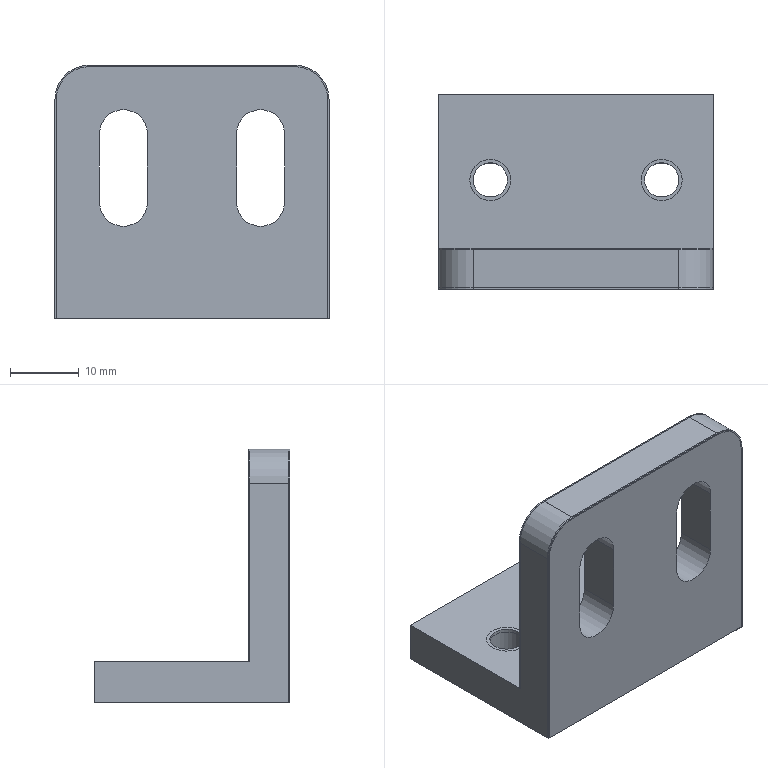NC program | NX | posted with a generic post | part box 40 x 28.5 x 37 mm
Lines 1 to 1288 of 1837:
N10 G17 G21 G94 G90
(PLANAR_MILL_1 , TOOL : D6.)
N12 T05 M6
N14 G53
N16 G17 G0 G90 X25.936 Y10.48 B0. C0. S2500 M3
N18 G43 Z50. H5
N20 Z-22.2 B-180.
N22 G94 G1 X16.946 Z-22.31 F1200.
N24 X16.82 Y10.448 Z-22.311
N26 X16.707 Y10.384 Z-22.313
N28 X16.616 Y10.293 Z-22.315
N30 X16.552 Y10.18 Z-22.316
N32 X16.52 Y10.054 Z-22.318
N34 Y9.946 Z-22.319
N36 X16.552 Y9.82 Z-22.321
N38 X16.616 Y9.707 Z-22.322
N40 X16.707 Y9.616 Z-22.324
N42 X16.82 Y9.552 Z-22.325
N44 X16.946 Y9.52 Z-22.327
N46 X27.054 Z-22.45
N48 X27.18 Y9.552 Z-22.452
N50 X27.293 Y9.616 Z-22.454
N52 X27.384 Y9.707 Z-22.455
N54 X27.448 Y9.82 Z-22.457
N56 X27.48 Y9.946 Z-22.458
N58 Y10.054 Z-22.46
N60 X27.448 Y10.18 Z-22.461
N62 X27.384 Y10.293 Z-22.463
N64 X27.293 Y10.384 Z-22.464
N66 X27.18 Y10.448 Z-22.466
N68 X27.054 Y10.48 Z-22.468
N70 X16.946 Z-22.591
N72 X16.82 Y10.448 Z-22.593
N74 X16.707 Y10.384 Z-22.594
N76 X16.616 Y10.293 Z-22.596
N78 X16.552 Y10.18 Z-22.598
N80 X16.52 Y10.054 Z-22.599
N82 Y9.946 Z-22.6
N84 X16.552 Y9.82 Z-22.602
N86 X16.616 Y9.707 Z-22.604
N88 X16.707 Y9.616 Z-22.605
N90 X16.82 Y9.552 Z-22.607
N92 X16.946 Y9.52 Z-22.608
N94 X27.054 Z-22.732
N96 X27.18 Y9.552 Z-22.733
N98 X27.293 Y9.616 Z-22.735
N100 X27.384 Y9.707 Z-22.737
N102 X27.448 Y9.82 Z-22.738
N104 X27.48 Y9.946 Z-22.74
N106 Y10.054 Z-22.741
N108 X27.448 Y10.18 Z-22.743
N110 X27.384 Y10.293 Z-22.744
N112 X27.293 Y10.384 Z-22.746
N114 X27.18 Y10.448 Z-22.747
N116 X27.054 Y10.48 Z-22.749
N118 X16.946 Z-22.872
N120 X16.82 Y10.448 Z-22.874
N122 X16.707 Y10.384 Z-22.876
N124 X16.616 Y10.293 Z-22.877
N126 X16.552 Y10.18 Z-22.879
N128 X16.52 Y10.054 Z-22.88
N130 Y9.946 Z-22.882
N132 X16.552 Y9.82 Z-22.883
N134 X16.616 Y9.707 Z-22.885
N136 X16.707 Y9.616 Z-22.886
N138 X16.82 Y9.552 Z-22.888
N140 X16.946 Y9.52 Z-22.89
N142 X27.054 Z-23.013
N144 X27.18 Y9.552 Z-23.015
N146 X27.293 Y9.616 Z-23.016
N148 X27.384 Y9.707 Z-23.018
N150 X27.448 Y9.82 Z-23.02
N152 X27.48 Y9.946 Z-23.021
N154 Y10.054 Z-23.022
N156 X27.448 Y10.18 Z-23.024
N158 X27.384 Y10.293 Z-23.026
N160 X27.293 Y10.384 Z-23.027
N162 X27.18 Y10.448 Z-23.029
N164 X27.054 Y10.48 Z-23.03
N166 X16.946 Z-23.154
N168 X16.82 Y10.448 Z-23.155
N170 X16.707 Y10.384 Z-23.157
N172 X16.616 Y10.293 Z-23.159
N174 X16.552 Y10.18 Z-23.16
N176 X16.52 Y10.054 Z-23.162
N178 Y9.946 Z-23.163
N180 X16.552 Y9.82 Z-23.165
N182 X16.616 Y9.707 Z-23.166
N184 X16.707 Y9.616 Z-23.168
N186 X16.82 Y9.552 Z-23.169
N188 X16.946 Y9.52 Z-23.171
N190 X27.054 Z-23.294
N192 X27.18 Y9.552 Z-23.296
N194 X27.293 Y9.616 Z-23.298
N196 X27.384 Y9.707 Z-23.299
N198 X27.448 Y9.82 Z-23.301
N200 X27.48 Y9.946 Z-23.302
N202 Y10.054 Z-23.304
N204 X27.448 Y10.18 Z-23.305
N206 X27.384 Y10.293 Z-23.307
N208 X27.293 Y10.384 Z-23.308
N210 X27.18 Y10.448 Z-23.31
N212 X27.054 Y10.48 Z-23.312
N214 X16.946 Z-23.435
N216 X16.82 Y10.448 Z-23.437
N218 X16.707 Y10.384 Z-23.438
N220 X16.616 Y10.293 Z-23.44
N222 X16.552 Y10.18 Z-23.441
N224 X16.52 Y10.054 Z-23.443
N226 Y9.946 Z-23.444
N228 X16.552 Y9.82 Z-23.446
N230 X16.616 Y9.707 Z-23.448
N232 X16.707 Y9.616 Z-23.449
N234 X16.82 Y9.552 Z-23.451
N236 X16.946 Y9.52 Z-23.452
N238 X27.054 Z-23.576
N240 X27.18 Y9.552 Z-23.577
N242 X27.293 Y9.616 Z-23.579
N244 X27.384 Y9.707 Z-23.581
N246 X27.448 Y9.82 Z-23.582
N248 X27.48 Y9.946 Z-23.584
N250 Y10.054 Z-23.585
N252 X27.448 Y10.18 Z-23.587
N254 X27.384 Y10.293 Z-23.588
N256 X27.293 Y10.384 Z-23.59
N258 X27.18 Y10.448 Z-23.591
N260 X27.054 Y10.48 Z-23.593
N262 X16.946 Z-23.716
N264 X16.82 Y10.448 Z-23.718
N266 X16.707 Y10.384 Z-23.72
N268 X16.616 Y10.293 Z-23.721
N270 X16.552 Y10.18 Z-23.723
N272 X16.52 Y10.054 Z-23.724
N274 Y9.946 Z-23.726
N276 X16.552 Y9.82 Z-23.727
N278 X16.616 Y9.707 Z-23.729
N280 X16.707 Y9.616 Z-23.73
N282 X16.82 Y9.552 Z-23.732
N284 X16.946 Y9.52 Z-23.734
N286 X27.054 Z-23.857
N288 X27.18 Y9.552 Z-23.859
N290 X27.293 Y9.616 Z-23.86
N292 X27.384 Y9.707 Z-23.862
N294 X27.448 Y9.82 Z-23.863
N296 X27.48 Y9.946 Z-23.865
N298 Y10.054 Z-23.866
N300 X27.448 Y10.18 Z-23.868
N302 X27.384 Y10.293 Z-23.87
N304 X27.293 Y10.384 Z-23.871
N306 X27.18 Y10.448 Z-23.873
N308 X27.054 Y10.48 Z-23.874
N310 X16.946 Z-23.998
N312 X16.82 Y10.448 Z-23.999
N314 X16.707 Y10.384 Z-24.001
N316 X16.616 Y10.293 Z-24.003
N318 X16.552 Y10.18 Z-24.004
N320 X16.52 Y10.054 Z-24.006
N322 Y9.946 Z-24.007
N324 X16.552 Y9.82 Z-24.009
N326 X16.616 Y9.707 Z-24.01
N328 X16.707 Y9.616 Z-24.012
N330 X16.82 Y9.552 Z-24.013
N332 X16.946 Y9.52 Z-24.015
N334 X27.054 Z-24.138
N336 X27.18 Y9.552 Z-24.14
N338 X27.293 Y9.616 Z-24.142
N340 X27.384 Y9.707 Z-24.143
N342 X27.448 Y9.82 Z-24.145
N344 X27.48 Y9.946 Z-24.146
N346 Y10.054 Z-24.148
N348 X27.448 Y10.18 Z-24.149
N350 X27.384 Y10.293 Z-24.151
N352 X27.293 Y10.384 Z-24.152
N354 X27.18 Y10.448 Z-24.154
N356 X27.054 Y10.48 Z-24.156
N358 X16.946 Z-24.279
N360 X16.82 Y10.448 Z-24.281
N362 X16.707 Y10.384 Z-24.282
N364 X16.616 Y10.293 Z-24.284
N366 X16.552 Y10.18 Z-24.285
N368 X16.52 Y10.054 Z-24.287
N370 Y9.946 Z-24.288
N372 X16.552 Y9.82 Z-24.29
N374 X16.616 Y9.707 Z-24.292
N376 X16.707 Y9.616 Z-24.293
N378 X16.82 Y9.552 Z-24.295
N380 X16.946 Y9.52 Z-24.296
N382 X27.054 Z-24.42
N384 X27.18 Y9.552 Z-24.421
N386 X27.293 Y9.616 Z-24.423
N388 X27.384 Y9.707 Z-24.425
N390 X27.448 Y9.82 Z-24.426
N392 X27.48 Y9.946 Z-24.428
N394 Y10.054 Z-24.429
N396 X27.448 Y10.18 Z-24.431
N398 X27.384 Y10.293 Z-24.432
N400 X27.293 Y10.384 Z-24.434
N402 X27.18 Y10.448 Z-24.435
N404 X27.054 Y10.48 Z-24.437
N406 X16.946 Z-24.56
N408 X16.82 Y10.448 Z-24.562
N410 X16.707 Y10.384 Z-24.564
N412 X16.616 Y10.293 Z-24.565
N414 X16.552 Y10.18 Z-24.567
N416 X16.52 Y10.054 Z-24.568
N418 Y9.946 Z-24.57
N420 X16.552 Y9.82 Z-24.571
N422 X16.616 Y9.707 Z-24.573
N424 X16.707 Y9.616 Z-24.574
N426 X16.82 Y9.552 Z-24.576
N428 X16.946 Y9.52 Z-24.578
N430 X27.054 Z-24.701
N432 X27.18 Y9.552 Z-24.703
N434 X27.293 Y9.616 Z-24.704
N436 X27.384 Y9.707 Z-24.706
N438 X27.448 Y9.82 Z-24.707
N440 X27.48 Y9.946 Z-24.709
N442 Y10.054 Z-24.71
N444 X27.448 Y10.18 Z-24.712
N446 X27.384 Y10.293 Z-24.714
N448 X27.293 Y10.384 Z-24.715
N450 X27.18 Y10.448 Z-24.717
N452 X27.054 Y10.48 Z-24.718
N454 X16.946 Z-24.842
N456 X16.82 Y10.448 Z-24.843
N458 X16.707 Y10.384 Z-24.845
N460 X16.616 Y10.293 Z-24.847
N462 X16.552 Y10.18 Z-24.848
N464 X16.52 Y10.054 Z-24.85
N466 Y9.946 Z-24.851
N468 X16.552 Y9.82 Z-24.853
N470 X16.616 Y9.707 Z-24.854
N472 X16.707 Y9.616 Z-24.856
N474 X16.82 Y9.552 Z-24.857
N476 X16.946 Y9.52 Z-24.859
N478 X27.054 Z-24.982
N480 X27.18 Y9.552 Z-24.984
N482 X27.293 Y9.616 Z-24.986
N484 X27.384 Y9.707 Z-24.987
N486 X27.448 Y9.82 Z-24.989
N488 X27.48 Y9.946 Z-24.99
N490 Y10.054 Z-24.992
N492 X27.448 Y10.18 Z-24.993
N494 X27.384 Y10.293 Z-24.995
N496 X27.293 Y10.384 Z-24.996
N498 X27.18 Y10.448 Z-24.998
N500 X27.054 Y10.48 Z-25.
N502 X16.946 Z-25.123
N504 X16.82 Y10.448 Z-25.125
N506 X16.707 Y10.384 Z-25.126
N508 X16.616 Y10.293 Z-25.128
N510 X16.552 Y10.18 Z-25.129
N512 X16.52 Y10.054 Z-25.131
N514 Y9.946 Z-25.132
N516 X16.552 Y9.82 Z-25.134
N518 X16.616 Y9.707 Z-25.136
N520 X16.707 Y9.616 Z-25.137
N522 X16.82 Y9.552 Z-25.139
N524 X16.946 Y9.52 Z-25.14
N526 X27.054 Z-25.264
N528 X27.18 Y9.552 Z-25.265
N530 X27.293 Y9.616 Z-25.267
N532 X27.384 Y9.707 Z-25.269
N534 X27.448 Y9.82 Z-25.27
N536 X27.48 Y9.946 Z-25.272
N538 Y10.054 Z-25.273
N540 X27.448 Y10.18 Z-25.275
N542 X27.384 Y10.293 Z-25.276
N544 X27.293 Y10.384 Z-25.278
N546 X27.18 Y10.448 Z-25.279
N548 X27.054 Y10.48 Z-25.281
N550 X16.946 Z-25.404
N552 X16.82 Y10.448 Z-25.406
N554 X16.707 Y10.384 Z-25.408
N556 X16.616 Y10.293 Z-25.409
N558 X16.552 Y10.18 Z-25.411
N560 X16.52 Y10.054 Z-25.412
N562 Y9.946 Z-25.414
N564 X16.552 Y9.82 Z-25.415
N566 X16.616 Y9.707 Z-25.417
N568 X16.707 Y9.616 Z-25.418
N570 X16.82 Y9.552 Z-25.42
N572 X16.946 Y9.52 Z-25.422
N574 X27.054 Z-25.545
N576 X27.18 Y9.552 Z-25.547
N578 X27.293 Y9.616 Z-25.548
N580 X27.384 Y9.707 Z-25.55
N582 X27.448 Y9.82 Z-25.551
N584 X27.48 Y9.946 Z-25.553
N586 Y10.054 Z-25.554
N588 X27.448 Y10.18 Z-25.556
N590 X27.384 Y10.293 Z-25.558
N592 X27.293 Y10.384 Z-25.559
N594 X27.18 Y10.448 Z-25.561
N596 X27.054 Y10.48 Z-25.562
N598 X16.946 Z-25.686
N600 X16.82 Y10.448 Z-25.687
N602 X16.707 Y10.384 Z-25.689
N604 X16.616 Y10.293 Z-25.691
N606 X16.552 Y10.18 Z-25.692
N608 X16.52 Y10.054 Z-25.694
N610 Y9.946 Z-25.695
N612 X16.552 Y9.82 Z-25.697
N614 X16.616 Y9.707 Z-25.698
N616 X16.707 Y9.616 Z-25.7
N618 X16.82 Y9.552 Z-25.701
N620 X16.946 Y9.52 Z-25.703
N622 X27.054 Z-25.826
N624 X27.18 Y9.552 Z-25.828
N626 X27.293 Y9.616 Z-25.83
N628 X27.384 Y9.707 Z-25.831
N630 X27.448 Y9.82 Z-25.833
N632 X27.48 Y9.946 Z-25.834
N634 Y10.054 Z-25.836
N636 X27.448 Y10.18 Z-25.837
N638 X27.384 Y10.293 Z-25.839
N640 X27.293 Y10.384 Z-25.84
N642 X27.18 Y10.448 Z-25.842
N644 X27.054 Y10.48 Z-25.844
N646 X16.946 Z-25.967
N648 X16.82 Y10.448 Z-25.969
N650 X16.707 Y10.384 Z-25.97
N652 X16.616 Y10.293 Z-25.972
N654 X16.552 Y10.18 Z-25.973
N656 X16.52 Y10.054 Z-25.975
N658 Y9.946 Z-25.976
N660 X16.552 Y9.82 Z-25.978
N662 X16.616 Y9.707 Z-25.98
N664 X16.707 Y9.616 Z-25.981
N666 X16.82 Y9.552 Z-25.983
N668 X16.946 Y9.52 Z-25.984
N670 X27.054 Z-26.108
N672 X27.18 Y9.552 Z-26.109
N674 X27.293 Y9.616 Z-26.111
N676 X27.384 Y9.707 Z-26.113
N678 X27.448 Y9.82 Z-26.114
N680 X27.48 Y9.946 Z-26.116
N682 Y10.054 Z-26.117
N684 X27.448 Y10.18 Z-26.119
N686 X27.384 Y10.293 Z-26.12
N688 X27.293 Y10.384 Z-26.122
N690 X27.18 Y10.448 Z-26.123
N692 X27.054 Y10.48 Z-26.125
N694 X16.946 Z-26.248
N696 X16.82 Y10.448 Z-26.25
N698 X16.707 Y10.384 Z-26.252
N700 X16.616 Y10.293 Z-26.253
N702 X16.552 Y10.18 Z-26.255
N704 X16.52 Y10.054 Z-26.256
N706 Y9.946 Z-26.258
N708 X16.552 Y9.82 Z-26.259
N710 X16.616 Y9.707 Z-26.261
N712 X16.707 Y9.616 Z-26.262
N714 X16.82 Y9.552 Z-26.264
N716 X16.946 Y9.52 Z-26.266
N718 X27.054 Z-26.389
N720 X27.18 Y9.552 Z-26.391
N722 X27.293 Y9.616 Z-26.392
N724 X27.384 Y9.707 Z-26.394
N726 X27.448 Y9.82 Z-26.395
N728 X27.48 Y9.946 Z-26.397
N730 Y10.054 Z-26.398
N732 X27.448 Y10.18 Z-26.4
N734 X27.384 Y10.293 Z-26.402
N736 X27.293 Y10.384 Z-26.403
N738 X27.18 Y10.448 Z-26.405
N740 X27.054 Y10.48 Z-26.406
N742 X16.946 Z-26.53
N744 X16.82 Y10.448 Z-26.531
N746 X16.707 Y10.384 Z-26.533
N748 X16.616 Y10.293 Z-26.535
N750 X16.552 Y10.18 Z-26.536
N752 X16.52 Y10.054 Z-26.538
N754 Y9.946 Z-26.539
N756 X16.552 Y9.82 Z-26.541
N758 X16.616 Y9.707 Z-26.542
N760 X16.707 Y9.616 Z-26.544
N762 X16.82 Y9.552 Z-26.545
N764 X16.946 Y9.52 Z-26.547
N766 X27.054 Z-26.67
N768 X27.18 Y9.552 Z-26.672
N770 X27.293 Y9.616 Z-26.674
N772 X27.384 Y9.707 Z-26.675
N774 X27.448 Y9.82 Z-26.677
N776 X27.48 Y9.946 Z-26.678
N778 Y10.054 Z-26.68
N780 X27.448 Y10.18 Z-26.681
N782 X27.384 Y10.293 Z-26.683
N784 X27.293 Y10.384 Z-26.684
N786 X27.18 Y10.448 Z-26.686
N788 X27.054 Y10.48 Z-26.688
N790 X16.946 Z-26.811
N792 X16.82 Y10.448 Z-26.813
N794 X16.707 Y10.384 Z-26.814
N796 X16.616 Y10.293 Z-26.816
N798 X16.552 Y10.18 Z-26.817
N800 X16.52 Y10.054 Z-26.819
N802 Y9.946 Z-26.82
N804 X16.552 Y9.82 Z-26.822
N806 X16.616 Y9.707 Z-26.824
N808 X16.707 Y9.616 Z-26.825
N810 X16.82 Y9.552 Z-26.827
N812 X16.946 Y9.52 Z-26.828
N814 X27.054 Z-26.952
N816 X27.18 Y9.552 Z-26.953
N818 X27.293 Y9.616 Z-26.955
N820 X27.384 Y9.707 Z-26.957
N822 X27.448 Y9.82 Z-26.958
N824 X27.48 Y9.946 Z-26.96
N826 Y10.054 Z-26.961
N828 X27.448 Y10.18 Z-26.963
N830 X27.384 Y10.293 Z-26.964
N832 X27.293 Y10.384 Z-26.966
N834 X27.18 Y10.448 Z-26.967
N836 X27.054 Y10.48 Z-26.969
N838 X16.946 Z-27.092
N840 X16.82 Y10.448 Z-27.094
N842 X16.707 Y10.384 Z-27.096
N844 X16.616 Y10.293 Z-27.097
N846 X16.552 Y10.18 Z-27.099
N848 X16.52 Y10.054 Z-27.1
N850 Y9.946 Z-27.102
N852 X16.552 Y9.82 Z-27.103
N854 X16.616 Y9.707 Z-27.105
N856 X16.707 Y9.616 Z-27.106
N858 X16.82 Y9.552 Z-27.108
N860 X16.946 Y9.52 Z-27.11
N862 X27.054 Z-27.233
N864 X27.18 Y9.552 Z-27.235
N866 X27.293 Y9.616 Z-27.236
N868 X27.384 Y9.707 Z-27.238
N870 X27.448 Y9.82 Z-27.239
N872 X27.48 Y9.946 Z-27.241
N874 Y10.054 Z-27.242
N876 X27.448 Y10.18 Z-27.244
N878 X27.384 Y10.293 Z-27.246
N880 X27.293 Y10.384 Z-27.247
N882 X27.18 Y10.448 Z-27.249
N884 X27.054 Y10.48 Z-27.25
N886 X16.946 Z-27.374
N888 X16.82 Y10.448 Z-27.375
N890 X16.707 Y10.384 Z-27.377
N892 X16.616 Y10.293 Z-27.379
N894 X16.552 Y10.18 Z-27.38
N896 X16.52 Y10.054 Z-27.382
N898 Y9.946 Z-27.383
N900 X16.552 Y9.82 Z-27.385
N902 X16.616 Y9.707 Z-27.386
N904 X16.707 Y9.616 Z-27.388
N906 X16.82 Y9.552 Z-27.389
N908 X16.946 Y9.52 Z-27.391
N910 X27.054 Z-27.514
N912 X27.18 Y9.552 Z-27.516
N914 X27.293 Y9.616 Z-27.518
N916 X27.384 Y9.707 Z-27.519
N918 X27.448 Y9.82 Z-27.521
N920 X27.48 Y9.946 Z-27.522
N922 Y10.054 Z-27.524
N924 X27.448 Y10.18 Z-27.525
N926 X27.384 Y10.293 Z-27.527
N928 X27.293 Y10.384 Z-27.528
N930 X27.18 Y10.448 Z-27.53
N932 X27.054 Y10.48 Z-27.532
N934 X16.946 Z-27.655
N936 X16.82 Y10.448 Z-27.657
N938 X16.707 Y10.384 Z-27.658
N940 X16.616 Y10.293 Z-27.66
N942 X16.552 Y10.18 Z-27.661
N944 X16.52 Y10.054 Z-27.663
N946 Y9.946 Z-27.664
N948 X16.552 Y9.82 Z-27.666
N950 X16.616 Y9.707 Z-27.668
N952 X16.707 Y9.616 Z-27.669
N954 X16.82 Y9.552 Z-27.671
N956 X16.946 Y9.52 Z-27.672
N958 X27.054 Z-27.796
N960 X27.18 Y9.552 Z-27.797
N962 X27.293 Y9.616 Z-27.799
N964 X27.384 Y9.707 Z-27.801
N966 X27.448 Y9.82 Z-27.802
N968 X27.48 Y9.946 Z-27.804
N970 Y10.054 Z-27.805
N972 X27.448 Y10.18 Z-27.807
N974 X27.384 Y10.293 Z-27.808
N976 X27.293 Y10.384 Z-27.81
N978 X27.18 Y10.448 Z-27.811
N980 X27.054 Y10.48 Z-27.813
N982 X16.946 Z-27.936
N984 X16.82 Y10.448 Z-27.938
N986 X16.707 Y10.384 Z-27.94
N988 X16.616 Y10.293 Z-27.941
N990 X16.552 Y10.18 Z-27.943
N992 X16.52 Y10.054 Z-27.944
N994 Y9.946 Z-27.946
N996 X16.552 Y9.82 Z-27.947
N998 X16.616 Y9.707 Z-27.949
N1000 X16.707 Y9.616 Z-27.95
N1002 X16.82 Y9.552 Z-27.952
N1004 X16.946 Y9.52 Z-27.954
N1006 X27.054 Z-28.077
N1008 X27.18 Y9.552 Z-28.079
N1010 X27.293 Y9.616 Z-28.08
N1012 X27.384 Y9.707 Z-28.082
N1014 X27.448 Y9.82 Z-28.083
N1016 X27.48 Y9.946 Z-28.085
N1018 Y10.054 Z-28.086
N1020 X27.448 Y10.18 Z-28.088
N1022 X27.384 Y10.293 Z-28.09
N1024 X27.293 Y10.384 Z-28.091
N1026 X27.18 Y10.448 Z-28.093
N1028 X27.054 Y10.48 Z-28.094
N1030 X16.946 Z-28.218
N1032 X16.82 Y10.448 Z-28.219
N1034 X16.707 Y10.384 Z-28.221
N1036 X16.616 Y10.293 Z-28.223
N1038 X16.552 Y10.18 Z-28.224
N1040 X16.52 Y10.054 Z-28.226
N1042 Y9.946 Z-28.227
N1044 X16.552 Y9.82 Z-28.229
N1046 X16.616 Y9.707 Z-28.23
N1048 X16.707 Y9.616 Z-28.232
N1050 X16.82 Y9.552 Z-28.233
N1052 X16.946 Y9.52 Z-28.235
N1054 X27.054 Z-28.358
N1056 X27.18 Y9.552 Z-28.36
N1058 X27.293 Y9.616 Z-28.362
N1060 X27.384 Y9.707 Z-28.363
N1062 X27.448 Y9.82 Z-28.365
N1064 X27.48 Y9.946 Z-28.366
N1066 Y10.054 Z-28.368
N1068 X27.448 Y10.18 Z-28.369
N1070 X27.384 Y10.293 Z-28.371
N1072 X27.293 Y10.384 Z-28.372
N1074 X27.18 Y10.448 Z-28.374
N1076 X27.054 Y10.48 Z-28.376
N1078 X16.946 Z-28.499
N1080 X16.82 Y10.448 Z-28.501
N1082 X16.707 Y10.384 Z-28.502
N1084 X16.616 Y10.293 Z-28.504
N1086 X16.552 Y10.18 Z-28.505
N1088 X16.52 Y10.054 Z-28.507
N1090 Y9.946 Z-28.508
N1092 X16.552 Y9.82 Z-28.51
N1094 X16.616 Y9.707 Z-28.512
N1096 X16.707 Y9.616 Z-28.513
N1098 X16.82 Y9.552 Z-28.515
N1100 X16.946 Y9.52 Z-28.516
N1102 X27.054 Z-28.64
N1104 X27.18 Y9.552 Z-28.641
N1106 X27.293 Y9.616 Z-28.643
N1108 X27.384 Y9.707 Z-28.645
N1110 X27.448 Y9.82 Z-28.646
N1112 X27.48 Y9.946 Z-28.648
N1114 Y10.054 Z-28.649
N1116 X27.448 Y10.18 Z-28.651
N1118 X27.384 Y10.293 Z-28.652
N1120 X27.293 Y10.384 Z-28.654
N1122 X27.18 Y10.448 Z-28.655
N1124 X27.054 Y10.48 Z-28.657
N1126 X16.946 Z-28.78
N1128 X16.82 Y10.448 Z-28.782
N1130 X16.707 Y10.384 Z-28.784
N1132 X16.616 Y10.293 Z-28.785
N1134 X16.552 Y10.18 Z-28.787
N1136 X16.52 Y10.054 Z-28.788
N1138 Y9.946 Z-28.79
N1140 X16.552 Y9.82 Z-28.791
N1142 X16.616 Y9.707 Z-28.793
N1144 X16.707 Y9.616 Z-28.794
N1146 X16.82 Y9.552 Z-28.796
N1148 X16.946 Y9.52 Z-28.798
N1150 X27.054 Z-28.921
N1152 X27.18 Y9.552 Z-28.923
N1154 X27.293 Y9.616 Z-28.924
N1156 X27.384 Y9.707 Z-28.926
N1158 X27.448 Y9.82 Z-28.927
N1160 X27.48 Y9.946 Z-28.929
N1162 Y10.054 Z-28.93
N1164 X27.448 Y10.18 Z-28.932
N1166 X27.384 Y10.293 Z-28.933
N1168 X27.293 Y10.384 Z-28.935
N1170 X27.18 Y10.448 Z-28.937
N1172 X27.054 Y10.48 Z-28.938
N1174 X22. Z-29.
N1176 X17.
N1178 G3 X16.52 Y10. R0.48
N1180 X17. Y9.52 R0.48
N1182 G1 X27.
N1184 G3 X27.48 Y10. R0.48
N1186 X27. Y10.48 R0.48
N1188 G1 X22.
N1190 X21.949 Y10.469
N1192 X21.911 Y10.432
N1194 X21.9 Y10.38
N1196 Z-26.
N1198 G0 Z50.
N1200 X25.936 Y-9.52
N1202 Z-22.2
N1204 G1 X16.946 Z-22.31
N1206 X16.82 Y-9.552 Z-22.311
N1208 X16.707 Y-9.616 Z-22.313
N1210 X16.616 Y-9.707 Z-22.315
N1212 X16.552 Y-9.82 Z-22.316
N1214 X16.52 Y-9.946 Z-22.318
N1216 Y-10.054 Z-22.319
N1218 X16.552 Y-10.18 Z-22.321
N1220 X16.616 Y-10.293 Z-22.322
N1222 X16.707 Y-10.384 Z-22.324
N1224 X16.82 Y-10.448 Z-22.325
N1226 X16.946 Y-10.48 Z-22.327
N1228 X27.054 Z-22.45
N1230 X27.18 Y-10.448 Z-22.452
N1232 X27.293 Y-10.384 Z-22.454
N1234 X27.384 Y-10.293 Z-22.455
N1236 X27.448 Y-10.18 Z-22.457
N1238 X27.48 Y-10.054 Z-22.458
N1240 Y-9.946 Z-22.46
N1242 X27.448 Y-9.82 Z-22.461
N1244 X27.384 Y-9.707 Z-22.463
N1246 X27.293 Y-9.616 Z-22.464
N1248 X27.18 Y-9.552 Z-22.466
N1250 X27.054 Y-9.52 Z-22.468
N1252 X16.946 Z-22.591
N1254 X16.82 Y-9.552 Z-22.593
N1256 X16.707 Y-9.616 Z-22.594
N1258 X16.616 Y-9.707 Z-22.596
N1260 X16.552 Y-9.82 Z-22.598
N1262 X16.52 Y-9.946 Z-22.599
N1264 Y-10.054 Z-22.6
N1266 X16.552 Y-10.18 Z-22.602
N1268 X16.616 Y-10.293 Z-22.604
N1270 X16.707 Y-10.384 Z-22.605
N1272 X16.82 Y-10.448 Z-22.607
N1274 X16.946 Y-10.48 Z-22.608
N1276 X27.054 Z-22.732
N1278 X27.18 Y-10.448 Z-22.733
N1280 X27.293 Y-10.384 Z-22.735
N1282 X27.384 Y-10.293 Z-22.737
N1284 X27.448 Y-10.18 Z-22.738
N1286 X27.48 Y-10.054 Z-22.74
N1288 Y-9.946 Z-22.741
N1290 X27.448 Y-9.82 Z-22.743
N1292 X27.384 Y-9.707 Z-22.744
N1294 X27.293 Y-9.616 Z-22.746
N1296 X27.18 Y-9.552 Z-22.747
N1298 X27.054 Y-9.52 Z-22.749
N1300 X16.946 Z-22.872
N1302 X16.82 Y-9.552 Z-22.874
N1304 X16.707 Y-9.616 Z-22.876
N1306 X16.616 Y-9.707 Z-22.877
N1308 X16.552 Y-9.82 Z-22.879
N1310 X16.52 Y-9.946 Z-22.88
N1312 Y-10.054 Z-22.882
N1314 X16.552 Y-10.18 Z-22.883
N1316 X16.616 Y-10.293 Z-22.885
N1318 X16.707 Y-10.384 Z-22.886
N1320 X16.82 Y-10.448 Z-22.888
N1322 X16.946 Y-10.48 Z-22.89
N1324 X27.054 Z-23.013
N1326 X27.18 Y-10.448 Z-23.015
N1328 X27.293 Y-10.384 Z-23.016
N1330 X27.384 Y-10.293 Z-23.018
N1332 X27.448 Y-10.18 Z-23.02
N1334 X27.48 Y-10.054 Z-23.021
N1336 Y-9.946 Z-23.022
N1338 X27.448 Y-9.82 Z-23.024
N1340 X27.384 Y-9.707 Z-23.026
N1342 X27.293 Y-9.616 Z-23.027
N1344 X27.18 Y-9.552 Z-23.029
N1346 X27.054 Y-9.52 Z-23.03
N1348 X16.946 Z-23.154
N1350 X16.82 Y-9.552 Z-23.155
N1352 X16.707 Y-9.616 Z-23.157
N1354 X16.616 Y-9.707 Z-23.159
N1356 X16.552 Y-9.82 Z-23.16
N1358 X16.52 Y-9.946 Z-23.162
N1360 Y-10.054 Z-23.163
N1362 X16.552 Y-10.18 Z-23.165
N1364 X16.616 Y-10.293 Z-23.166
N1366 X16.707 Y-10.384 Z-23.168
N1368 X16.82 Y-10.448 Z-23.169
N1370 X16.946 Y-10.48 Z-23.171
N1372 X27.054 Z-23.294
N1374 X27.18 Y-10.448 Z-23.296
N1376 X27.293 Y-10.384 Z-23.298
N1378 X27.384 Y-10.293 Z-23.299
N1380 X27.448 Y-10.18 Z-23.301
N1382 X27.48 Y-10.054 Z-23.302
N1384 Y-9.946 Z-23.304
N1386 X27.448 Y-9.82 Z-23.305
N1388 X27.384 Y-9.707 Z-23.307
N1390 X27.293 Y-9.616 Z-23.308
N1392 X27.18 Y-9.552 Z-23.31
N1394 X27.054 Y-9.52 Z-23.312
N1396 X16.946 Z-23.435
N1398 X16.82 Y-9.552 Z-23.437
N1400 X16.707 Y-9.616 Z-23.438
N1402 X16.616 Y-9.707 Z-23.44
N1404 X16.552 Y-9.82 Z-23.441
N1406 X16.52 Y-9.946 Z-23.443
N1408 Y-10.054 Z-23.444
N1410 X16.552 Y-10.18 Z-23.446
N1412 X16.616 Y-10.293 Z-23.448
N1414 X16.707 Y-10.384 Z-23.449
N1416 X16.82 Y-10.448 Z-23.451
N1418 X16.946 Y-10.48 Z-23.452
N1420 X27.054 Z-23.576
N1422 X27.18 Y-10.448 Z-23.577
N1424 X27.293 Y-10.384 Z-23.579
N1426 X27.384 Y-10.293 Z-23.581
N1428 X27.448 Y-10.18 Z-23.582
N1430 X27.48 Y-10.054 Z-23.584
N1432 Y-9.946 Z-23.585
N1434 X27.448 Y-9.82 Z-23.587
N1436 X27.384 Y-9.707 Z-23.588
N1438 X27.293 Y-9.616 Z-23.59
N1440 X27.18 Y-9.552 Z-23.591
N1442 X27.054 Y-9.52 Z-23.593
N1444 X16.946 Z-23.716
N1446 X16.82 Y-9.552 Z-23.718
N1448 X16.707 Y-9.616 Z-23.72
N1450 X16.616 Y-9.707 Z-23.721
N1452 X16.552 Y-9.82 Z-23.723
N1454 X16.52 Y-9.946 Z-23.724
N1456 Y-10.054 Z-23.726
N1458 X16.552 Y-10.18 Z-23.727
N1460 X16.616 Y-10.293 Z-23.729
N1462 X16.707 Y-10.384 Z-23.73
N1464 X16.82 Y-10.448 Z-23.732
N1466 X16.946 Y-10.48 Z-23.734
N1468 X27.054 Z-23.857
N1470 X27.18 Y-10.448 Z-23.859
N1472 X27.293 Y-10.384 Z-23.86
N1474 X27.384 Y-10.293 Z-23.862
N1476 X27.448 Y-10.18 Z-23.863
N1478 X27.48 Y-10.054 Z-23.865
N1480 Y-9.946 Z-23.866
N1482 X27.448 Y-9.82 Z-23.868
N1484 X27.384 Y-9.707 Z-23.87
N1486 X27.293 Y-9.616 Z-23.871
N1488 X27.18 Y-9.552 Z-23.873
N1490 X27.054 Y-9.52 Z-23.874
N1492 X16.946 Z-23.998
N1494 X16.82 Y-9.552 Z-23.999
N1496 X16.707 Y-9.616 Z-24.001
N1498 X16.616 Y-9.707 Z-24.003
N1500 X16.552 Y-9.82 Z-24.004
N1502 X16.52 Y-9.946 Z-24.006
N1504 Y-10.054 Z-24.007
N1506 X16.552 Y-10.18 Z-24.009
N1508 X16.616 Y-10.293 Z-24.01
N1510 X16.707 Y-10.384 Z-24.012
N1512 X16.82 Y-10.448 Z-24.013
N1514 X16.946 Y-10.48 Z-24.015
N1516 X27.054 Z-24.138
N1518 X27.18 Y-10.448 Z-24.14
N1520 X27.293 Y-10.384 Z-24.142
N1522 X27.384 Y-10.293 Z-24.143
N1524 X27.448 Y-10.18 Z-24.145
N1526 X27.48 Y-10.054 Z-24.146
N1528 Y-9.946 Z-24.148
N1530 X27.448 Y-9.82 Z-24.149
N1532 X27.384 Y-9.707 Z-24.151
N1534 X27.293 Y-9.616 Z-24.152
N1536 X27.18 Y-9.552 Z-24.154
N1538 X27.054 Y-9.52 Z-24.156
N1540 X16.946 Z-24.279
N1542 X16.82 Y-9.552 Z-24.281
N1544 X16.707 Y-9.616 Z-24.282
N1546 X16.616 Y-9.707 Z-24.284
N1548 X16.552 Y-9.82 Z-24.285
N1550 X16.52 Y-9.946 Z-24.287
N1552 Y-10.054 Z-24.288
N1554 X16.552 Y-10.18 Z-24.29
N1556 X16.616 Y-10.293 Z-24.292
N1558 X16.707 Y-10.384 Z-24.293
N1560 X16.82 Y-10.448 Z-24.295
N1562 X16.946 Y-10.48 Z-24.296
N1564 X27.054 Z-24.42
N1566 X27.18 Y-10.448 Z-24.421
N1568 X27.293 Y-10.384 Z-24.423
N1570 X27.384 Y-10.293 Z-24.425
N1572 X27.448 Y-10.18 Z-24.426
N1574 X27.48 Y-10.054 Z-24.428
N1576 Y-9.946 Z-24.429
N1578 X27.448 Y-9.82 Z-24.431
N1580 X27.384 Y-9.707 Z-24.432
N1582 X27.293 Y-9.616 Z-24.434
N1584 X27.18 Y-9.552 Z-24.435
N1586 X27.054 Y-9.52 Z-24.437
N1588 X16.946 Z-24.56
N1590 X16.82 Y-9.552 Z-24.562
N1592 X16.707 Y-9.616 Z-24.564
N1594 X16.616 Y-9.707 Z-24.565
N1596 X16.552 Y-9.82 Z-24.567
N1598 X16.52 Y-9.946 Z-24.568
N1600 Y-10.054 Z-24.57
N1602 X16.552 Y-10.18 Z-24.571
N1604 X16.616 Y-10.293 Z-24.573
N1606 X16.707 Y-10.384 Z-24.574
N1608 X16.82 Y-10.448 Z-24.576
N1610 X16.946 Y-10.48 Z-24.578
N1612 X27.054 Z-24.701
N1614 X27.18 Y-10.448 Z-24.703
N1616 X27.293 Y-10.384 Z-24.704
N1618 X27.384 Y-10.293 Z-24.706
N1620 X27.448 Y-10.18 Z-24.707
N1622 X27.48 Y-10.054 Z-24.709
N1624 Y-9.946 Z-24.71
N1626 X27.448 Y-9.82 Z-24.712
N1628 X27.384 Y-9.707 Z-24.714
N1630 X27.293 Y-9.616 Z-24.715
N1632 X27.18 Y-9.552 Z-24.717
N1634 X27.054 Y-9.52 Z-24.718
N1636 X16.946 Z-24.842
N1638 X16.82 Y-9.552 Z-24.843
N1640 X16.707 Y-9.616 Z-24.845
N1642 X16.616 Y-9.707 Z-24.847
N1644 X16.552 Y-9.82 Z-24.848
N1646 X16.52 Y-9.946 Z-24.85
N1648 Y-10.054 Z-24.851
N1650 X16.552 Y-10.18 Z-24.853
N1652 X16.616 Y-10.293 Z-24.854
N1654 X16.707 Y-10.384 Z-24.856
N1656 X16.82 Y-10.448 Z-24.857
N1658 X16.946 Y-10.48 Z-24.859
N1660 X27.054 Z-24.982
N1662 X27.18 Y-10.448 Z-24.984
N1664 X27.293 Y-10.384 Z-24.986
N1666 X27.384 Y-10.293 Z-24.987
N1668 X27.448 Y-10.18 Z-24.989
N1670 X27.48 Y-10.054 Z-24.99
N1672 Y-9.946 Z-24.992
N1674 X27.448 Y-9.82 Z-24.993
N1676 X27.384 Y-9.707 Z-24.995
N1678 X27.293 Y-9.616 Z-24.996
N1680 X27.18 Y-9.552 Z-24.998
N1682 X27.054 Y-9.52 Z-25.
N1684 X16.946 Z-25.123
N1686 X16.82 Y-9.552 Z-25.125
N1688 X16.707 Y-9.616 Z-25.126
N1690 X16.616 Y-9.707 Z-25.128
N1692 X16.552 Y-9.82 Z-25.129
N1694 X16.52 Y-9.946 Z-25.131
N1696 Y-10.054 Z-25.132
N1698 X16.552 Y-10.18 Z-25.134
N1700 X16.616 Y-10.293 Z-25.136
N1702 X16.707 Y-10.384 Z-25.137
N1704 X16.82 Y-10.448 Z-25.139
N1706 X16.946 Y-10.48 Z-25.14
N1708 X27.054 Z-25.264
N1710 X27.18 Y-10.448 Z-25.265
N1712 X27.293 Y-10.384 Z-25.267
N1714 X27.384 Y-10.293 Z-25.269
N1716 X27.448 Y-10.18 Z-25.27
N1718 X27.48 Y-10.054 Z-25.272
N1720 Y-9.946 Z-25.273
N1722 X27.448 Y-9.82 Z-25.275
N1724 X27.384 Y-9.707 Z-25.276
N1726 X27.293 Y-9.616 Z-25.278
N1728 X27.18 Y-9.552 Z-25.279
N1730 X27.054 Y-9.52 Z-25.281
N1732 X16.946 Z-25.404
N1734 X16.82 Y-9.552 Z-25.406
N1736 X16.707 Y-9.616 Z-25.408
N1738 X16.616 Y-9.707 Z-25.409
N1740 X16.552 Y-9.82 Z-25.411
N1742 X16.52 Y-9.946 Z-25.412
N1744 Y-10.054 Z-25.414
N1746 X16.552 Y-10.18 Z-25.415
N1748 X16.616 Y-10.293 Z-25.417
N1750 X16.707 Y-10.384 Z-25.418
N1752 X16.82 Y-10.448 Z-25.42
N1754 X16.946 Y-10.48 Z-25.422
N1756 X27.054 Z-25.545
N1758 X27.18 Y-10.448 Z-25.547
N1760 X27.293 Y-10.384 Z-25.548
N1762 X27.384 Y-10.293 Z-25.55
N1764 X27.448 Y-10.18 Z-25.551
N1766 X27.48 Y-10.054 Z-25.553
N1768 Y-9.946 Z-25.554
N1770 X27.448 Y-9.82 Z-25.556
N1772 X27.384 Y-9.707 Z-25.558
N1774 X27.293 Y-9.616 Z-25.559
N1776 X27.18 Y-9.552 Z-25.561
N1778 X27.054 Y-9.52 Z-25.562
N1780 X16.946 Z-25.686
N1782 X16.82 Y-9.552 Z-25.687
N1784 X16.707 Y-9.616 Z-25.689
N1786 X16.616 Y-9.707 Z-25.691
N1788 X16.552 Y-9.82 Z-25.692
N1790 X16.52 Y-9.946 Z-25.694
N1792 Y-10.054 Z-25.695
N1794 X16.552 Y-10.18 Z-25.697
N1796 X16.616 Y-10.293 Z-25.698
N1798 X16.707 Y-10.384 Z-25.7
N1800 X16.82 Y-10.448 Z-25.701
N1802 X16.946 Y-10.48 Z-25.703
N1804 X27.054 Z-25.826
N1806 X27.18 Y-10.448 Z-25.828
N1808 X27.293 Y-10.384 Z-25.83
N1810 X27.384 Y-10.293 Z-25.831
N1812 X27.448 Y-10.18 Z-25.833
N1814 X27.48 Y-10.054 Z-25.834
N1816 Y-9.946 Z-25.836
N1818 X27.448 Y-9.82 Z-25.837
N1820 X27.384 Y-9.707 Z-25.839
N1822 X27.293 Y-9.616 Z-25.84
N1824 X27.18 Y-9.552 Z-25.842
N1826 X27.054 Y-9.52 Z-25.844
N1828 X16.946 Z-25.967
N1830 X16.82 Y-9.552 Z-25.969
N1832 X16.707 Y-9.616 Z-25.97
N1834 X16.616 Y-9.707 Z-25.972
N1836 X16.552 Y-9.82 Z-25.973
N1838 X16.52 Y-9.946 Z-25.975
N1840 Y-10.054 Z-25.976
N1842 X16.552 Y-10.18 Z-25.978
N1844 X16.616 Y-10.293 Z-25.98
N1846 X16.707 Y-10.384 Z-25.981
N1848 X16.82 Y-10.448 Z-25.983
N1850 X16.946 Y-10.48 Z-25.984
N1852 X27.054 Z-26.108
N1854 X27.18 Y-10.448 Z-26.109
N1856 X27.293 Y-10.384 Z-26.111
N1858 X27.384 Y-10.293 Z-26.113
N1860 X27.448 Y-10.18 Z-26.114
N1862 X27.48 Y-10.054 Z-26.116
N1864 Y-9.946 Z-26.117
N1866 X27.448 Y-9.82 Z-26.119
N1868 X27.384 Y-9.707 Z-26.12
N1870 X27.293 Y-9.616 Z-26.122
N1872 X27.18 Y-9.552 Z-26.123
N1874 X27.054 Y-9.52 Z-26.125
N1876 X16.946 Z-26.248
N1878 X16.82 Y-9.552 Z-26.25
N1880 X16.707 Y-9.616 Z-26.252
N1882 X16.616 Y-9.707 Z-26.253
N1884 X16.552 Y-9.82 Z-26.255
N1886 X16.52 Y-9.946 Z-26.256
N1888 Y-10.054 Z-26.258
N1890 X16.552 Y-10.18 Z-26.259
N1892 X16.616 Y-10.293 Z-26.261
N1894 X16.707 Y-10.384 Z-26.262
N1896 X16.82 Y-10.448 Z-26.264
N1898 X16.946 Y-10.48 Z-26.266
N1900 X27.054 Z-26.389
N1902 X27.18 Y-10.448 Z-26.391
N1904 X27.293 Y-10.384 Z-26.392
N1906 X27.384 Y-10.293 Z-26.394
N1908 X27.448 Y-10.18 Z-26.395
N1910 X27.48 Y-10.054 Z-26.397
N1912 Y-9.946 Z-26.398
N1914 X27.448 Y-9.82 Z-26.4
N1916 X27.384 Y-9.707 Z-26.402
N1918 X27.293 Y-9.616 Z-26.403
N1920 X27.18 Y-9.552 Z-26.405
N1922 X27.054 Y-9.52 Z-26.406
N1924 X16.946 Z-26.53
N1926 X16.82 Y-9.552 Z-26.531
N1928 X16.707 Y-9.616 Z-26.533
N1930 X16.616 Y-9.707 Z-26.535
N1932 X16.552 Y-9.82 Z-26.536
N1934 X16.52 Y-9.946 Z-26.538
N1936 Y-10.054 Z-26.539
N1938 X16.552 Y-10.18 Z-26.541
N1940 X16.616 Y-10.293 Z-26.542
N1942 X16.707 Y-10.384 Z-26.544
N1944 X16.82 Y-10.448 Z-26.545
N1946 X16.946 Y-10.48 Z-26.547
N1948 X27.054 Z-26.67
N1950 X27.18 Y-10.448 Z-26.672
N1952 X27.293 Y-10.384 Z-26.674
N1954 X27.384 Y-10.293 Z-26.675
N1956 X27.448 Y-10.18 Z-26.677
N1958 X27.48 Y-10.054 Z-26.678
N1960 Y-9.946 Z-26.68
N1962 X27.448 Y-9.82 Z-26.681
N1964 X27.384 Y-9.707 Z-26.683
N1966 X27.293 Y-9.616 Z-26.684
N1968 X27.18 Y-9.552 Z-26.686
N1970 X27.054 Y-9.52 Z-26.688
N1972 X16.946 Z-26.811
N1974 X16.82 Y-9.552 Z-26.813
N1976 X16.707 Y-9.616 Z-26.814
N1978 X16.616 Y-9.707 Z-26.816
N1980 X16.552 Y-9.82 Z-26.817
N1982 X16.52 Y-9.946 Z-26.819
N1984 Y-10.054 Z-26.82
N1986 X16.552 Y-10.18 Z-26.822
N1988 X16.616 Y-10.293 Z-26.824
N1990 X16.707 Y-10.384 Z-26.825
N1992 X16.82 Y-10.448 Z-26.827
N1994 X16.946 Y-10.48 Z-26.828
N1996 X27.054 Z-26.952
N1998 X27.18 Y-10.448 Z-26.953
N2000 X27.293 Y-10.384 Z-26.955
N2002 X27.384 Y-10.293 Z-26.957
N2004 X27.448 Y-10.18 Z-26.958
N2006 X27.48 Y-10.054 Z-26.96
N2008 Y-9.946 Z-26.961
N2010 X27.448 Y-9.82 Z-26.963
N2012 X27.384 Y-9.707 Z-26.964
N2014 X27.293 Y-9.616 Z-26.966
N2016 X27.18 Y-9.552 Z-26.967
N2018 X27.054 Y-9.52 Z-26.969
N2020 X16.946 Z-27.092
N2022 X16.82 Y-9.552 Z-27.094
N2024 X16.707 Y-9.616 Z-27.096
N2026 X16.616 Y-9.707 Z-27.097
N2028 X16.552 Y-9.82 Z-27.099
N2030 X16.52 Y-9.946 Z-27.1
N2032 Y-10.054 Z-27.102
N2034 X16.552 Y-10.18 Z-27.103
N2036 X16.616 Y-10.293 Z-27.105
N2038 X16.707 Y-10.384 Z-27.106
N2040 X16.82 Y-10.448 Z-27.108
N2042 X16.946 Y-10.48 Z-27.11
N2044 X27.054 Z-27.233
N2046 X27.18 Y-10.448 Z-27.235
N2048 X27.293 Y-10.384 Z-27.236
N2050 X27.384 Y-10.293 Z-27.238
N2052 X27.448 Y-10.18 Z-27.239
N2054 X27.48 Y-10.054 Z-27.241
N2056 Y-9.946 Z-27.242
N2058 X27.448 Y-9.82 Z-27.244
N2060 X27.384 Y-9.707 Z-27.246
N2062 X27.293 Y-9.616 Z-27.247
N2064 X27.18 Y-9.552 Z-27.249
N2066 X27.054 Y-9.52 Z-27.25
N2068 X16.946 Z-27.374
N2070 X16.82 Y-9.552 Z-27.375
N2072 X16.707 Y-9.616 Z-27.377
N2074 X16.616 Y-9.707 Z-27.379
N2076 X16.552 Y-9.82 Z-27.38
N2078 X16.52 Y-9.946 Z-27.382
N2080 Y-10.054 Z-27.383
N2082 X16.552 Y-10.18 Z-27.385
N2084 X16.616 Y-10.293 Z-27.386
N2086 X16.707 Y-10.384 Z-27.388
N2088 X16.82 Y-10.448 Z-27.389
N2090 X16.946 Y-10.48 Z-27.391
N2092 X27.054 Z-27.514
N2094 X27.18 Y-10.448 Z-27.516
N2096 X27.293 Y-10.384 Z-27.518
N2098 X27.384 Y-10.293 Z-27.519
N2100 X27.448 Y-10.18 Z-27.521
N2102 X27.48 Y-10.054 Z-27.522
N2104 Y-9.946 Z-27.524
N2106 X27.448 Y-9.82 Z-27.525
N2108 X27.384 Y-9.707 Z-27.527
N2110 X27.293 Y-9.616 Z-27.528
N2112 X27.18 Y-9.552 Z-27.53
N2114 X27.054 Y-9.52 Z-27.532
N2116 X16.946 Z-27.655
N2118 X16.82 Y-9.552 Z-27.657
N2120 X16.707 Y-9.616 Z-27.658
N2122 X16.616 Y-9.707 Z-27.66
N2124 X16.552 Y-9.82 Z-27.661
N2126 X16.52 Y-9.946 Z-27.663
N2128 Y-10.054 Z-27.664
N2130 X16.552 Y-10.18 Z-27.666
N2132 X16.616 Y-10.293 Z-27.668
N2134 X16.707 Y-10.384 Z-27.669
N2136 X16.82 Y-10.448 Z-27.671
N2138 X16.946 Y-10.48 Z-27.672
N2140 X27.054 Z-27.796
N2142 X27.18 Y-10.448 Z-27.797
N2144 X27.293 Y-10.384 Z-27.799
N2146 X27.384 Y-10.293 Z-27.801
N2148 X27.448 Y-10.18 Z-27.802
N2150 X27.48 Y-10.054 Z-27.804
N2152 Y-9.946 Z-27.805
N2154 X27.448 Y-9.82 Z-27.807
N2156 X27.384 Y-9.707 Z-27.808
N2158 X27.293 Y-9.616 Z-27.81
N2160 X27.18 Y-9.552 Z-27.811
N2162 X27.054 Y-9.52 Z-27.813
N2164 X16.946 Z-27.936
N2166 X16.82 Y-9.552 Z-27.938
N2168 X16.707 Y-9.616 Z-27.94
N2170 X16.616 Y-9.707 Z-27.941
N2172 X16.552 Y-9.82 Z-27.943
N2174 X16.52 Y-9.946 Z-27.944
N2176 Y-10.054 Z-27.946
N2178 X16.552 Y-10.18 Z-27.947
N2180 X16.616 Y-10.293 Z-27.949
N2182 X16.707 Y-10.384 Z-27.95
N2184 X16.82 Y-10.448 Z-27.952
N2186 X16.946 Y-10.48 Z-27.954
N2188 X27.054 Z-28.077
N2190 X27.18 Y-10.448 Z-28.079
N2192 X27.293 Y-10.384 Z-28.08
N2194 X27.384 Y-10.293 Z-28.082
N2196 X27.448 Y-10.18 Z-28.083
N2198 X27.48 Y-10.054 Z-28.085
N2200 Y-9.946 Z-28.086
N2202 X27.448 Y-9.82 Z-28.088
N2204 X27.384 Y-9.707 Z-28.09
N2206 X27.293 Y-9.616 Z-28.091
N2208 X27.18 Y-9.552 Z-28.093
N2210 X27.054 Y-9.52 Z-28.094
N2212 X16.946 Z-28.218
N2214 X16.82 Y-9.552 Z-28.219
N2216 X16.707 Y-9.616 Z-28.221
N2218 X16.616 Y-9.707 Z-28.223
N2220 X16.552 Y-9.82 Z-28.224
N2222 X16.52 Y-9.946 Z-28.226
N2224 Y-10.054 Z-28.227
N2226 X16.552 Y-10.18 Z-28.229
N2228 X16.616 Y-10.293 Z-28.23
N2230 X16.707 Y-10.384 Z-28.232
N2232 X16.82 Y-10.448 Z-28.233
N2234 X16.946 Y-10.48 Z-28.235
N2236 X27.054 Z-28.358
N2238 X27.18 Y-10.448 Z-28.36
N2240 X27.293 Y-10.384 Z-28.362
N2242 X27.384 Y-10.293 Z-28.363
N2244 X27.448 Y-10.18 Z-28.365
N2246 X27.48 Y-10.054 Z-28.366
N2248 Y-9.946 Z-28.368
N2250 X27.448 Y-9.82 Z-28.369
N2252 X27.384 Y-9.707 Z-28.371
N2254 X27.293 Y-9.616 Z-28.372
N2256 X27.18 Y-9.552 Z-28.374
N2258 X27.054 Y-9.52 Z-28.376
N2260 X16.946 Z-28.499
N2262 X16.82 Y-9.552 Z-28.501
N2264 X16.707 Y-9.616 Z-28.502
N2266 X16.616 Y-9.707 Z-28.504
N2268 X16.552 Y-9.82 Z-28.505
N2270 X16.52 Y-9.946 Z-28.507
N2272 Y-10.054 Z-28.508
N2274 X16.552 Y-10.18 Z-28.51
N2276 X16.616 Y-10.293 Z-28.512
N2278 X16.707 Y-10.384 Z-28.513
N2280 X16.82 Y-10.448 Z-28.515
N2282 X16.946 Y-10.48 Z-28.516
N2284 X27.054 Z-28.64
N2286 X27.18 Y-10.448 Z-28.641
N2288 X27.293 Y-10.384 Z-28.643
N2290 X27.384 Y-10.293 Z-28.645
N2292 X27.448 Y-10.18 Z-28.646
N2294 X27.48 Y-10.054 Z-28.648
N2296 Y-9.946 Z-28.649
N2298 X27.448 Y-9.82 Z-28.651
N2300 X27.384 Y-9.707 Z-28.652
N2302 X27.293 Y-9.616 Z-28.654
N2304 X27.18 Y-9.552 Z-28.655
N2306 X27.054 Y-9.52 Z-28.657
N2308 X16.946 Z-28.78
N2310 X16.82 Y-9.552 Z-28.782
N2312 X16.707 Y-9.616 Z-28.784
N2314 X16.616 Y-9.707 Z-28.785
N2316 X16.552 Y-9.82 Z-28.787
N2318 X16.52 Y-9.946 Z-28.788
N2320 Y-10.054 Z-28.79
N2322 X16.552 Y-10.18 Z-28.791
N2324 X16.616 Y-10.293 Z-28.793
N2326 X16.707 Y-10.384 Z-28.794
N2328 X16.82 Y-10.448 Z-28.796
N2330 X16.946 Y-10.48 Z-28.798
N2332 X27.054 Z-28.921
N2334 X27.18 Y-10.448 Z-28.923
N2336 X27.293 Y-10.384 Z-28.924
N2338 X27.384 Y-10.293 Z-28.926
N2340 X27.448 Y-10.18 Z-28.927
N2342 X27.48 Y-10.054 Z-28.929
N2344 Y-9.946 Z-28.93
N2346 X27.448 Y-9.82 Z-28.932
N2348 X27.384 Y-9.707 Z-28.933
N2350 X27.293 Y-9.616 Z-28.935
N2352 X27.18 Y-9.552 Z-28.937
N2354 X27.054 Y-9.52 Z-28.938
N2356 X22. Z-29.
N2358 X17.
N2360 G3 X16.52 Y-10. R0.48
N2362 X17. Y-10.48 R0.48
N2364 G1 X27.
N2366 G3 X27.48 Y-10. R0.48
N2368 X27. Y-9.52 R0.48
N2370 G1 X22.
N2372 X21.949 Y-9.531
N2374 X21.911 Y-9.569
N2376 X21.9 Y-9.62
N2378 Z-26.
N2380 G0 Z50.
N2382 M5
(PLANAR_MILL_1_COPY , TOOL : D6J)
N2384 T06 M6
N2386 G53
N2388 G17 G0 G90 X17.2 Y10. B0. C0. S2000 M3
N2390 G43 Z50. H6
N2392 Z-29. B-180.
N2394 G94 G1 Y10.3 F150.
N2396 G3 X17. Y10.5 R0.2
N2398 X16.5 Y10. R0.5
N2400 X17. Y9.5 R0.5
N2402 G1 X27.
N2404 G3 X27.5 Y10. R0.5
N2406 X27. Y10.5 R0.5
N2408 G1 X17.
N2410 X16.949 Y10.489
N2412 X16.911 Y10.452
N2414 X16.9 Y10.4
N2416 X17.2 Y10.3
N2418 G3 X17. Y10.5 R0.2
N2420 X16.5 Y10. R0.5
N2422 X17. Y9.5 R0.5
N2424 G1 X27.
N2426 G3 X27.5 Y10. R0.5
N2428 X27. Y10.5 R0.5
N2430 G1 X17.
N2432 X16.949 Y10.489
N2434 X16.911 Y10.452
N2436 X16.9 Y10.4
N2438 X17. Y10.
N2440 Z-26.
N2442 G0 Z50.
N2444 X17.2 Y-10.
N2446 Z-29.
N2448 G1 Y-9.7
N2450 G3 X17. Y-9.5 R0.2
N2452 X16.5 Y-10. R0.5
N2454 X17. Y-10.5 R0.5
N2456 G1 X27.
N2458 G3 X27.5 Y-10. R0.5
N2460 X27. Y-9.5 R0.5
N2462 G1 X17.
N2464 X16.949 Y-9.511
N2466 X16.911 Y-9.549
N2468 X16.9 Y-9.6
N2470 X17.2 Y-9.7
N2472 G3 X17. Y-9.5 R0.2
N2474 X16.5 Y-10. R0.5
N2476 X17. Y-10.5 R0.5
N2478 G1 X27.
N2480 G3 X27.5 Y-10. R0.5
N2482 X27. Y-9.5 R0.5
N2484 G1 X17.
N2486 X16.949 Y-9.511
N2488 X16.911 Y-9.549
N2490 X16.9 Y-9.6
N2492 X17. Y-10.
N2494 Z-26.
N2496 G0 Z50.
N2498 M5
(PLANAR_MILL_COPY_COPY_1_1_COPY_COPY_COPY , TOOL : 4倒角)
N2500 T19 M6
N2502 G53
N2504 G17 G0 G90 X26.826 Y10.015 B0. C0. S4500 M3
N2506 G43 Z50. H19
N2508 Z-24. B-180.
N2510 G41 G94 G1 X27. Y11. F800. D19
N2512 Y12.
N2514 X17.
N2516 G3 X15. Y10. R2.
N2518 X17. Y8. R2.
N2520 G1 X27.
N2522 G3 X29. Y10. R2.
N2524 X27. Y12. R2.
N2526 G1 Y11.
N2528 G40
N2530 X27.174 Y10.015
N2532 G0 Z50.
N2534 X17.174 Y-10.015
N2536 Z-24.
N2538 G41 G1 X17. Y-11.
N2540 Y-12.
N2542 X27.
N2544 G3 X29. Y-10. R2.
N2546 X27. Y-8. R2.
N2548 G1 X17.
N2550 G3 X15. Y-10. R2.
N2552 X17. Y-12. R2.
N2554 G1 Y-11.
N2556 G40
N2558 X16.826 Y-10.015
N2560 G0 Z50.
N2562 M5